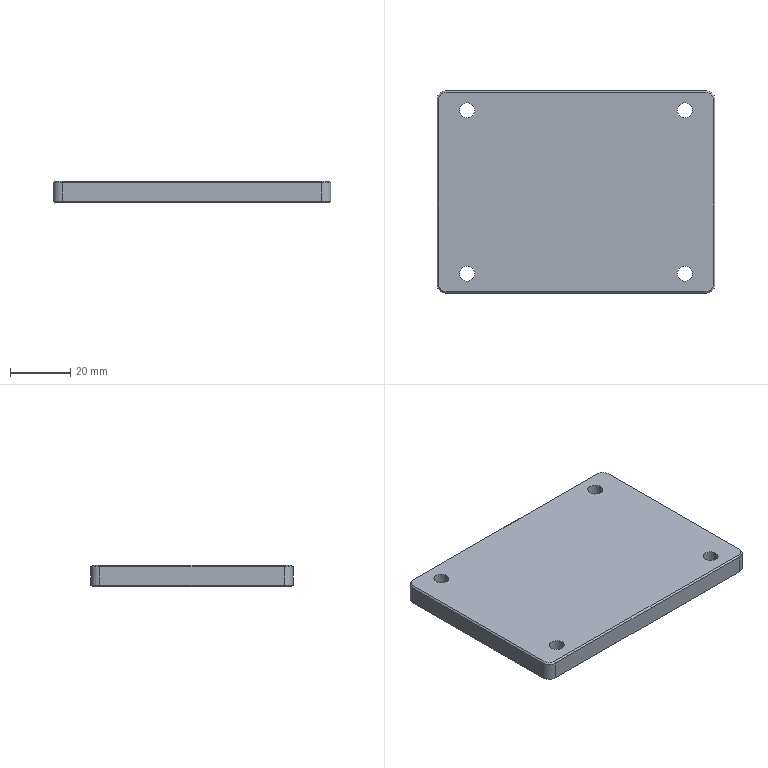Part | SolidWorks | features Chamfer 1, Extrusion 1, Fillet 1, ICE 1, LPattern 1 | 1 solid | 34 faces | box 92 x 67 x 7 mm | volume 42466 mm3 | plane 14 | cylinder 12 | cone 8 | commonest cylinder face diameters 5 x8 6 x4
STEP:
#1=CARTESIAN_POINT('',(38.5,27.,0.));
#2=VERTEX_POINT('',#1);
#3=CARTESIAN_POINT('',(33.5,27.,0.));
#4=VERTEX_POINT('',#3);
#5=CARTESIAN_POINT('',(36.,27.,0.));
#6=DIRECTION('',(0.,0.,-1.));
#7=DIRECTION('',(-1.,0.,0.));
#8=AXIS2_PLACEMENT_3D('',#5,#6,#7);
#9=CIRCLE('',#8,2.5);
#10=EDGE_CURVE('',#2,#4,#9,.T.);
#11=ORIENTED_EDGE('',*,*,#10,.T.);
#12=CARTESIAN_POINT('',(33.5,27.,7.));
#13=VERTEX_POINT('',#12);
#14=CARTESIAN_POINT('',(33.5,27.,-3.));
#15=DIRECTION('',(0.,0.,1.));
#16=VECTOR('',#15,1000.);
#17=LINE('',#14,#16);
#18=EDGE_CURVE('',#4,#13,#17,.T.);
#19=ORIENTED_EDGE('',*,*,#18,.T.);
#20=CARTESIAN_POINT('',(38.5,27.,7.));
#21=VERTEX_POINT('',#20);
#22=CARTESIAN_POINT('',(36.,27.,7.));
#23=DIRECTION('',(0.,0.,1.));
#24=DIRECTION('',(1.,0.,0.));
#25=AXIS2_PLACEMENT_3D('',#22,#23,#24);
#26=CIRCLE('',#25,2.5);
#27=EDGE_CURVE('',#13,#21,#26,.T.);
#28=ORIENTED_EDGE('',*,*,#27,.T.);
#29=CARTESIAN_POINT('',(38.5,27.,-3.));
#30=DIRECTION('',(0.,0.,1.));
#31=VECTOR('',#30,1000.);
#32=LINE('',#29,#31);
#33=EDGE_CURVE('',#2,#21,#32,.T.);
#34=ORIENTED_EDGE('',*,*,#33,.F.);
#35=EDGE_LOOP('',(#11,#19,#28,#34));
#36=FACE_OUTER_BOUND('',#35,.T.);
#37=CARTESIAN_POINT('',(36.,27.,-3.));
#38=DIRECTION('',(0.,0.,1.));
#39=DIRECTION('',(1.,0.,0.));
#40=AXIS2_PLACEMENT_3D('',#37,#38,#39);
#41=CYLINDRICAL_SURFACE('',#40,2.5);
#42=ADVANCED_FACE('',(#36),#41,.F.);
#43=CARTESIAN_POINT('',(-33.5,27.,0.));
#44=VERTEX_POINT('',#43);
#45=CARTESIAN_POINT('',(-38.5,27.,0.));
#46=VERTEX_POINT('',#45);
#47=CARTESIAN_POINT('',(-36.,27.,0.));
#48=DIRECTION('',(0.,0.,-1.));
#49=DIRECTION('',(-1.,0.,0.));
#50=AXIS2_PLACEMENT_3D('',#47,#48,#49);
#51=CIRCLE('',#50,2.5);
#52=EDGE_CURVE('',#44,#46,#51,.T.);
#53=ORIENTED_EDGE('',*,*,#52,.T.);
#54=CARTESIAN_POINT('',(-38.5,27.,7.));
#55=VERTEX_POINT('',#54);
#56=CARTESIAN_POINT('',(-38.5,27.,-3.));
#57=DIRECTION('',(0.,0.,1.));
#58=VECTOR('',#57,1000.);
#59=LINE('',#56,#58);
#60=EDGE_CURVE('',#46,#55,#59,.T.);
#61=ORIENTED_EDGE('',*,*,#60,.T.);
#62=CARTESIAN_POINT('',(-33.5,27.,7.));
#63=VERTEX_POINT('',#62);
#64=CARTESIAN_POINT('',(-36.,27.,7.));
#65=DIRECTION('',(0.,0.,1.));
#66=DIRECTION('',(1.,0.,0.));
#67=AXIS2_PLACEMENT_3D('',#64,#65,#66);
#68=CIRCLE('',#67,2.5);
#69=EDGE_CURVE('',#55,#63,#68,.T.);
#70=ORIENTED_EDGE('',*,*,#69,.T.);
#71=CARTESIAN_POINT('',(-33.5,27.,-3.));
#72=DIRECTION('',(0.,0.,1.));
#73=VECTOR('',#72,1000.);
#74=LINE('',#71,#73);
#75=EDGE_CURVE('',#44,#63,#74,.T.);
#76=ORIENTED_EDGE('',*,*,#75,.F.);
#77=EDGE_LOOP('',(#53,#61,#70,#76));
#78=FACE_OUTER_BOUND('',#77,.T.);
#79=CARTESIAN_POINT('',(-36.,27.,-3.));
#80=DIRECTION('',(0.,0.,1.));
#81=DIRECTION('',(1.,0.,0.));
#82=AXIS2_PLACEMENT_3D('',#79,#80,#81);
#83=CYLINDRICAL_SURFACE('',#82,2.5);
#84=ADVANCED_FACE('',(#78),#83,.F.);
#85=CARTESIAN_POINT('',(-33.5,-27.,0.));
#86=VERTEX_POINT('',#85);
#87=CARTESIAN_POINT('',(-38.5,-27.,0.));
#88=VERTEX_POINT('',#87);
#89=CARTESIAN_POINT('',(-36.,-27.,0.));
#90=DIRECTION('',(0.,0.,-1.));
#91=DIRECTION('',(-1.,0.,0.));
#92=AXIS2_PLACEMENT_3D('',#89,#90,#91);
#93=CIRCLE('',#92,2.5);
#94=EDGE_CURVE('',#86,#88,#93,.T.);
#95=ORIENTED_EDGE('',*,*,#94,.T.);
#96=CARTESIAN_POINT('',(-38.5,-27.,7.));
#97=VERTEX_POINT('',#96);
#98=CARTESIAN_POINT('',(-38.5,-27.,-3.));
#99=DIRECTION('',(0.,0.,1.));
#100=VECTOR('',#99,1000.);
#101=LINE('',#98,#100);
#102=EDGE_CURVE('',#88,#97,#101,.T.);
#103=ORIENTED_EDGE('',*,*,#102,.T.);
#104=CARTESIAN_POINT('',(-33.5,-27.,7.));
#105=VERTEX_POINT('',#104);
#106=CARTESIAN_POINT('',(-36.,-27.,7.));
#107=DIRECTION('',(0.,0.,1.));
#108=DIRECTION('',(1.,0.,0.));
#109=AXIS2_PLACEMENT_3D('',#106,#107,#108);
#110=CIRCLE('',#109,2.5);
#111=EDGE_CURVE('',#97,#105,#110,.T.);
#112=ORIENTED_EDGE('',*,*,#111,.T.);
#113=CARTESIAN_POINT('',(-33.5,-27.,-3.));
#114=DIRECTION('',(0.,0.,1.));
#115=VECTOR('',#114,1000.);
#116=LINE('',#113,#115);
#117=EDGE_CURVE('',#86,#105,#116,.T.);
#118=ORIENTED_EDGE('',*,*,#117,.F.);
#119=EDGE_LOOP('',(#95,#103,#112,#118));
#120=FACE_OUTER_BOUND('',#119,.T.);
#121=CARTESIAN_POINT('',(-36.,-27.,-3.));
#122=DIRECTION('',(0.,0.,1.));
#123=DIRECTION('',(1.,0.,0.));
#124=AXIS2_PLACEMENT_3D('',#121,#122,#123);
#125=CYLINDRICAL_SURFACE('',#124,2.5);
#126=ADVANCED_FACE('',(#120),#125,.F.);
#127=CARTESIAN_POINT('',(38.5,-27.,0.));
#128=VERTEX_POINT('',#127);
#129=CARTESIAN_POINT('',(33.5,-27.,0.));
#130=VERTEX_POINT('',#129);
#131=CARTESIAN_POINT('',(36.,-27.,0.));
#132=DIRECTION('',(0.,0.,-1.));
#133=DIRECTION('',(-1.,0.,0.));
#134=AXIS2_PLACEMENT_3D('',#131,#132,#133);
#135=CIRCLE('',#134,2.5);
#136=EDGE_CURVE('',#128,#130,#135,.T.);
#137=ORIENTED_EDGE('',*,*,#136,.T.);
#138=CARTESIAN_POINT('',(33.5,-27.,7.));
#139=VERTEX_POINT('',#138);
#140=CARTESIAN_POINT('',(33.5,-27.,-3.));
#141=DIRECTION('',(0.,0.,1.));
#142=VECTOR('',#141,1000.);
#143=LINE('',#140,#142);
#144=EDGE_CURVE('',#130,#139,#143,.T.);
#145=ORIENTED_EDGE('',*,*,#144,.T.);
#146=CARTESIAN_POINT('',(38.5,-27.,7.));
#147=VERTEX_POINT('',#146);
#148=CARTESIAN_POINT('',(36.,-27.,7.));
#149=DIRECTION('',(0.,0.,1.));
#150=DIRECTION('',(1.,0.,0.));
#151=AXIS2_PLACEMENT_3D('',#148,#149,#150);
#152=CIRCLE('',#151,2.5);
#153=EDGE_CURVE('',#139,#147,#152,.T.);
#154=ORIENTED_EDGE('',*,*,#153,.T.);
#155=CARTESIAN_POINT('',(38.5,-27.,-3.));
#156=DIRECTION('',(0.,0.,1.));
#157=VECTOR('',#156,1000.);
#158=LINE('',#155,#157);
#159=EDGE_CURVE('',#128,#147,#158,.T.);
#160=ORIENTED_EDGE('',*,*,#159,.F.);
#161=EDGE_LOOP('',(#137,#145,#154,#160));
#162=FACE_OUTER_BOUND('',#161,.T.);
#163=CARTESIAN_POINT('',(36.,-27.,-3.));
#164=DIRECTION('',(0.,0.,1.));
#165=DIRECTION('',(1.,0.,0.));
#166=AXIS2_PLACEMENT_3D('',#163,#164,#165);
#167=CYLINDRICAL_SURFACE('',#166,2.5);
#168=ADVANCED_FACE('',(#162),#167,.F.);
#169=ORIENTED_EDGE('',*,*,#144,.F.);
#170=CARTESIAN_POINT('',(36.,-27.,0.));
#171=DIRECTION('',(0.,0.,-1.));
#172=DIRECTION('',(-1.,0.,0.));
#173=AXIS2_PLACEMENT_3D('',#170,#171,#172);
#174=CIRCLE('',#173,2.5);
#175=EDGE_CURVE('',#130,#128,#174,.T.);
#176=ORIENTED_EDGE('',*,*,#175,.T.);
#177=ORIENTED_EDGE('',*,*,#159,.T.);
#178=CARTESIAN_POINT('',(36.,-27.,7.));
#179=DIRECTION('',(0.,0.,1.));
#180=DIRECTION('',(1.,0.,0.));
#181=AXIS2_PLACEMENT_3D('',#178,#179,#180);
#182=CIRCLE('',#181,2.5);
#183=EDGE_CURVE('',#147,#139,#182,.T.);
#184=ORIENTED_EDGE('',*,*,#183,.T.);
#185=EDGE_LOOP('',(#169,#176,#177,#184));
#186=FACE_OUTER_BOUND('',#185,.T.);
#187=CARTESIAN_POINT('',(36.,-27.,-3.));
#188=DIRECTION('',(0.,0.,1.));
#189=DIRECTION('',(1.,0.,0.));
#190=AXIS2_PLACEMENT_3D('',#187,#188,#189);
#191=CYLINDRICAL_SURFACE('',#190,2.5);
#192=ADVANCED_FACE('',(#186),#191,.F.);
#193=ORIENTED_EDGE('',*,*,#102,.F.);
#194=CARTESIAN_POINT('',(-36.,-27.,0.));
#195=DIRECTION('',(0.,0.,-1.));
#196=DIRECTION('',(-1.,0.,0.));
#197=AXIS2_PLACEMENT_3D('',#194,#195,#196);
#198=CIRCLE('',#197,2.5);
#199=EDGE_CURVE('',#88,#86,#198,.T.);
#200=ORIENTED_EDGE('',*,*,#199,.T.);
#201=ORIENTED_EDGE('',*,*,#117,.T.);
#202=CARTESIAN_POINT('',(-36.,-27.,7.));
#203=DIRECTION('',(0.,0.,1.));
#204=DIRECTION('',(1.,0.,0.));
#205=AXIS2_PLACEMENT_3D('',#202,#203,#204);
#206=CIRCLE('',#205,2.5);
#207=EDGE_CURVE('',#105,#97,#206,.T.);
#208=ORIENTED_EDGE('',*,*,#207,.T.);
#209=EDGE_LOOP('',(#193,#200,#201,#208));
#210=FACE_OUTER_BOUND('',#209,.T.);
#211=CARTESIAN_POINT('',(-36.,-27.,-3.));
#212=DIRECTION('',(0.,0.,1.));
#213=DIRECTION('',(1.,0.,0.));
#214=AXIS2_PLACEMENT_3D('',#211,#212,#213);
#215=CYLINDRICAL_SURFACE('',#214,2.5);
#216=ADVANCED_FACE('',(#210),#215,.F.);
#217=CARTESIAN_POINT('',(46.,-30.5,6.5));
#218=VERTEX_POINT('',#217);
#219=CARTESIAN_POINT('',(46.,-30.5,0.5));
#220=VERTEX_POINT('',#219);
#221=CARTESIAN_POINT('',(46.,-30.5,7.));
#222=DIRECTION('',(0.,0.,-1.));
#223=VECTOR('',#222,1000.);
#224=LINE('',#221,#223);
#225=EDGE_CURVE('',#218,#220,#224,.T.);
#226=ORIENTED_EDGE('',*,*,#225,.T.);
#227=CARTESIAN_POINT('',(46.,30.5,0.5));
#228=VERTEX_POINT('',#227);
#229=CARTESIAN_POINT('',(46.,30.5,0.5));
#230=DIRECTION('',(0.,1.,0.));
#231=VECTOR('',#230,1000.);
#232=LINE('',#229,#231);
#233=EDGE_CURVE('',#220,#228,#232,.T.);
#234=ORIENTED_EDGE('',*,*,#233,.T.);
#235=CARTESIAN_POINT('',(46.,30.5,6.5));
#236=VERTEX_POINT('',#235);
#237=CARTESIAN_POINT('',(46.,30.5,7.));
#238=DIRECTION('',(0.,0.,1.));
#239=VECTOR('',#238,1000.);
#240=LINE('',#237,#239);
#241=EDGE_CURVE('',#228,#236,#240,.T.);
#242=ORIENTED_EDGE('',*,*,#241,.T.);
#243=CARTESIAN_POINT('',(46.,-33.5,6.5));
#244=DIRECTION('',(0.,-1.,0.));
#245=VECTOR('',#244,1000.);
#246=LINE('',#243,#245);
#247=EDGE_CURVE('',#236,#218,#246,.T.);
#248=ORIENTED_EDGE('',*,*,#247,.T.);
#249=EDGE_LOOP('',(#226,#234,#242,#248));
#250=FACE_OUTER_BOUND('',#249,.T.);
#251=CARTESIAN_POINT('',(46.,-33.5,7.));
#252=DIRECTION('',(-1.,0.,0.));
#253=DIRECTION('',(0.,0.,1.));
#254=AXIS2_PLACEMENT_3D('',#251,#252,#253);
#255=PLANE('',#254);
#256=ADVANCED_FACE('',(#250),#255,.F.);
#257=CARTESIAN_POINT('',(43.,33.5,6.5));
#258=VERTEX_POINT('',#257);
#259=CARTESIAN_POINT('',(43.,33.5,0.5));
#260=VERTEX_POINT('',#259);
#261=CARTESIAN_POINT('',(43.,33.5,7.));
#262=DIRECTION('',(0.,0.,-1.));
#263=VECTOR('',#262,1000.);
#264=LINE('',#261,#263);
#265=EDGE_CURVE('',#258,#260,#264,.T.);
#266=ORIENTED_EDGE('',*,*,#265,.T.);
#267=CARTESIAN_POINT('',(-43.,33.5,0.5));
#268=VERTEX_POINT('',#267);
#269=CARTESIAN_POINT('',(-43.,33.5,0.5));
#270=DIRECTION('',(-1.,0.,0.));
#271=VECTOR('',#270,1000.);
#272=LINE('',#269,#271);
#273=EDGE_CURVE('',#260,#268,#272,.T.);
#274=ORIENTED_EDGE('',*,*,#273,.T.);
#275=CARTESIAN_POINT('',(-43.,33.5,6.5));
#276=VERTEX_POINT('',#275);
#277=CARTESIAN_POINT('',(-43.,33.5,7.));
#278=DIRECTION('',(0.,0.,1.));
#279=VECTOR('',#278,1000.);
#280=LINE('',#277,#279);
#281=EDGE_CURVE('',#268,#276,#280,.T.);
#282=ORIENTED_EDGE('',*,*,#281,.T.);
#283=CARTESIAN_POINT('',(-46.,33.5,6.5));
#284=DIRECTION('',(1.,0.,0.));
#285=VECTOR('',#284,1000.);
#286=LINE('',#283,#285);
#287=EDGE_CURVE('',#276,#258,#286,.T.);
#288=ORIENTED_EDGE('',*,*,#287,.T.);
#289=EDGE_LOOP('',(#266,#274,#282,#288));
#290=FACE_OUTER_BOUND('',#289,.T.);
#291=CARTESIAN_POINT('',(-46.,33.5,7.));
#292=DIRECTION('',(0.,-1.,0.));
#293=DIRECTION('',(0.,0.,-1.));
#294=AXIS2_PLACEMENT_3D('',#291,#292,#293);
#295=PLANE('',#294);
#296=ADVANCED_FACE('',(#290),#295,.F.);
#297=CARTESIAN_POINT('',(-46.,30.5,6.5));
#298=VERTEX_POINT('',#297);
#299=CARTESIAN_POINT('',(-46.,30.5,0.5));
#300=VERTEX_POINT('',#299);
#301=CARTESIAN_POINT('',(-46.,30.5,7.));
#302=DIRECTION('',(0.,0.,-1.));
#303=VECTOR('',#302,1000.);
#304=LINE('',#301,#303);
#305=EDGE_CURVE('',#298,#300,#304,.T.);
#306=ORIENTED_EDGE('',*,*,#305,.T.);
#307=CARTESIAN_POINT('',(-46.,-30.5,0.5));
#308=VERTEX_POINT('',#307);
#309=CARTESIAN_POINT('',(-46.,-30.5,0.5));
#310=DIRECTION('',(0.,-1.,0.));
#311=VECTOR('',#310,1000.);
#312=LINE('',#309,#311);
#313=EDGE_CURVE('',#300,#308,#312,.T.);
#314=ORIENTED_EDGE('',*,*,#313,.T.);
#315=CARTESIAN_POINT('',(-46.,-30.5,6.5));
#316=VERTEX_POINT('',#315);
#317=CARTESIAN_POINT('',(-46.,-30.5,7.));
#318=DIRECTION('',(0.,0.,1.));
#319=VECTOR('',#318,1000.);
#320=LINE('',#317,#319);
#321=EDGE_CURVE('',#308,#316,#320,.T.);
#322=ORIENTED_EDGE('',*,*,#321,.T.);
#323=CARTESIAN_POINT('',(-46.,-33.5,6.5));
#324=DIRECTION('',(0.,1.,0.));
#325=VECTOR('',#324,1000.);
#326=LINE('',#323,#325);
#327=EDGE_CURVE('',#316,#298,#326,.T.);
#328=ORIENTED_EDGE('',*,*,#327,.T.);
#329=EDGE_LOOP('',(#306,#314,#322,#328));
#330=FACE_OUTER_BOUND('',#329,.T.);
#331=CARTESIAN_POINT('',(-46.,-33.5,7.));
#332=DIRECTION('',(1.,0.,0.));
#333=DIRECTION('',(0.,0.,-1.));
#334=AXIS2_PLACEMENT_3D('',#331,#332,#333);
#335=PLANE('',#334);
#336=ADVANCED_FACE('',(#330),#335,.F.);
#337=CARTESIAN_POINT('',(-43.,-33.5,6.5));
#338=VERTEX_POINT('',#337);
#339=CARTESIAN_POINT('',(-43.,-33.5,0.5));
#340=VERTEX_POINT('',#339);
#341=CARTESIAN_POINT('',(-43.,-33.5,7.));
#342=DIRECTION('',(0.,0.,-1.));
#343=VECTOR('',#342,1000.);
#344=LINE('',#341,#343);
#345=EDGE_CURVE('',#338,#340,#344,.T.);
#346=ORIENTED_EDGE('',*,*,#345,.T.);
#347=CARTESIAN_POINT('',(43.,-33.5,0.5));
#348=VERTEX_POINT('',#347);
#349=CARTESIAN_POINT('',(43.,-33.5,0.5));
#350=DIRECTION('',(1.,0.,0.));
#351=VECTOR('',#350,1000.);
#352=LINE('',#349,#351);
#353=EDGE_CURVE('',#340,#348,#352,.T.);
#354=ORIENTED_EDGE('',*,*,#353,.T.);
#355=CARTESIAN_POINT('',(43.,-33.5,6.5));
#356=VERTEX_POINT('',#355);
#357=CARTESIAN_POINT('',(43.,-33.5,7.));
#358=DIRECTION('',(0.,0.,1.));
#359=VECTOR('',#358,1000.);
#360=LINE('',#357,#359);
#361=EDGE_CURVE('',#348,#356,#360,.T.);
#362=ORIENTED_EDGE('',*,*,#361,.T.);
#363=CARTESIAN_POINT('',(-46.,-33.5,6.5));
#364=DIRECTION('',(-1.,0.,0.));
#365=VECTOR('',#364,1000.);
#366=LINE('',#363,#365);
#367=EDGE_CURVE('',#356,#338,#366,.T.);
#368=ORIENTED_EDGE('',*,*,#367,.T.);
#369=EDGE_LOOP('',(#346,#354,#362,#368));
#370=FACE_OUTER_BOUND('',#369,.T.);
#371=CARTESIAN_POINT('',(-46.,-33.5,7.));
#372=DIRECTION('',(0.,1.,0.));
#373=DIRECTION('',(0.,0.,1.));
#374=AXIS2_PLACEMENT_3D('',#371,#372,#373);
#375=PLANE('',#374);
#376=ADVANCED_FACE('',(#370),#375,.F.);
#377=CARTESIAN_POINT('',(43.,-33.,7.));
#378=VERTEX_POINT('',#377);
#379=CARTESIAN_POINT('',(45.5,-30.5,7.));
#380=VERTEX_POINT('',#379);
#381=CARTESIAN_POINT('',(43.,-30.5,7.));
#382=DIRECTION('',(0.,0.,1.));
#383=DIRECTION('',(-1.,0.,0.));
#384=AXIS2_PLACEMENT_3D('',#381,#382,#383);
#385=CIRCLE('',#384,2.5);
#386=EDGE_CURVE('',#378,#380,#385,.T.);
#387=ORIENTED_EDGE('',*,*,#386,.T.);
#388=CARTESIAN_POINT('',(45.5,30.5,7.));
#389=VERTEX_POINT('',#388);
#390=CARTESIAN_POINT('',(45.5,0.,7.));
#391=DIRECTION('',(0.,1.,0.));
#392=VECTOR('',#391,1000.);
#393=LINE('',#390,#392);
#394=EDGE_CURVE('',#380,#389,#393,.T.);
#395=ORIENTED_EDGE('',*,*,#394,.T.);
#396=CARTESIAN_POINT('',(43.,33.,7.));
#397=VERTEX_POINT('',#396);
#398=CARTESIAN_POINT('',(43.,30.5,7.));
#399=DIRECTION('',(0.,0.,1.));
#400=DIRECTION('',(-1.,0.,0.));
#401=AXIS2_PLACEMENT_3D('',#398,#399,#400);
#402=CIRCLE('',#401,2.5);
#403=EDGE_CURVE('',#389,#397,#402,.T.);
#404=ORIENTED_EDGE('',*,*,#403,.T.);
#405=CARTESIAN_POINT('',(-43.,33.,7.));
#406=VERTEX_POINT('',#405);
#407=CARTESIAN_POINT('',(0.,33.,7.));
#408=DIRECTION('',(-1.,0.,0.));
#409=VECTOR('',#408,1000.);
#410=LINE('',#407,#409);
#411=EDGE_CURVE('',#397,#406,#410,.T.);
#412=ORIENTED_EDGE('',*,*,#411,.T.);
#413=CARTESIAN_POINT('',(-45.5,30.5,7.));
#414=VERTEX_POINT('',#413);
#415=CARTESIAN_POINT('',(-43.,30.5,7.));
#416=DIRECTION('',(0.,0.,1.));
#417=DIRECTION('',(-1.,0.,0.));
#418=AXIS2_PLACEMENT_3D('',#415,#416,#417);
#419=CIRCLE('',#418,2.5);
#420=EDGE_CURVE('',#406,#414,#419,.T.);
#421=ORIENTED_EDGE('',*,*,#420,.T.);
#422=CARTESIAN_POINT('',(-45.5,-30.5,7.));
#423=VERTEX_POINT('',#422);
#424=CARTESIAN_POINT('',(-45.5,0.,7.));
#425=DIRECTION('',(0.,-1.,0.));
#426=VECTOR('',#425,1000.);
#427=LINE('',#424,#426);
#428=EDGE_CURVE('',#414,#423,#427,.T.);
#429=ORIENTED_EDGE('',*,*,#428,.T.);
#430=CARTESIAN_POINT('',(-43.,-33.,7.));
#431=VERTEX_POINT('',#430);
#432=CARTESIAN_POINT('',(-43.,-30.5,7.));
#433=DIRECTION('',(0.,0.,1.));
#434=DIRECTION('',(-1.,0.,0.));
#435=AXIS2_PLACEMENT_3D('',#432,#433,#434);
#436=CIRCLE('',#435,2.5);
#437=EDGE_CURVE('',#423,#431,#436,.T.);
#438=ORIENTED_EDGE('',*,*,#437,.T.);
#439=CARTESIAN_POINT('',(0.,-33.,7.));
#440=DIRECTION('',(1.,0.,0.));
#441=VECTOR('',#440,1000.);
#442=LINE('',#439,#441);
#443=EDGE_CURVE('',#431,#378,#442,.T.);
#444=ORIENTED_EDGE('',*,*,#443,.T.);
#445=EDGE_LOOP('',(#387,#395,#404,#412,#421,#429,#438,#444));
#446=FACE_OUTER_BOUND('',#445,.T.);
#447=CARTESIAN_POINT('',(36.,27.,7.));
#448=DIRECTION('',(0.,0.,1.));
#449=DIRECTION('',(1.,0.,0.));
#450=AXIS2_PLACEMENT_3D('',#447,#448,#449);
#451=CIRCLE('',#450,2.5);
#452=EDGE_CURVE('',#21,#13,#451,.T.);
#453=ORIENTED_EDGE('',*,*,#452,.F.);
#454=ORIENTED_EDGE('',*,*,#27,.F.);
#455=EDGE_LOOP('',(#453,#454));
#456=FACE_BOUND('',#455,.T.);
#457=CARTESIAN_POINT('',(-36.,27.,7.));
#458=DIRECTION('',(0.,0.,1.));
#459=DIRECTION('',(1.,0.,0.));
#460=AXIS2_PLACEMENT_3D('',#457,#458,#459);
#461=CIRCLE('',#460,2.5);
#462=EDGE_CURVE('',#63,#55,#461,.T.);
#463=ORIENTED_EDGE('',*,*,#462,.F.);
#464=ORIENTED_EDGE('',*,*,#69,.F.);
#465=EDGE_LOOP('',(#463,#464));
#466=FACE_BOUND('',#465,.T.);
#467=ORIENTED_EDGE('',*,*,#207,.F.);
#468=ORIENTED_EDGE('',*,*,#111,.F.);
#469=EDGE_LOOP('',(#467,#468));
#470=FACE_BOUND('',#469,.T.);
#471=ORIENTED_EDGE('',*,*,#183,.F.);
#472=ORIENTED_EDGE('',*,*,#153,.F.);
#473=EDGE_LOOP('',(#471,#472));
#474=FACE_BOUND('',#473,.T.);
#475=CARTESIAN_POINT('',(0.,0.,7.));
#476=DIRECTION('',(0.,0.,-1.));
#477=DIRECTION('',(-1.,0.,0.));
#478=AXIS2_PLACEMENT_3D('',#475,#476,#477);
#479=PLANE('',#478);
#480=ADVANCED_FACE('',(#446,#456,#466,#470,#474),#479,.F.);
#481=CARTESIAN_POINT('',(43.,33.,0.));
#482=VERTEX_POINT('',#481);
#483=CARTESIAN_POINT('',(45.5,30.5,0.));
#484=VERTEX_POINT('',#483);
#485=CARTESIAN_POINT('',(43.,30.5,0.));
#486=DIRECTION('',(0.,0.,-1.));
#487=DIRECTION('',(-1.,0.,0.));
#488=AXIS2_PLACEMENT_3D('',#485,#486,#487);
#489=CIRCLE('',#488,2.5);
#490=EDGE_CURVE('',#482,#484,#489,.T.);
#491=ORIENTED_EDGE('',*,*,#490,.T.);
#492=CARTESIAN_POINT('',(45.5,-30.5,0.));
#493=VERTEX_POINT('',#492);
#494=CARTESIAN_POINT('',(45.5,-30.5,0.));
#495=DIRECTION('',(0.,-1.,0.));
#496=VECTOR('',#495,1000.);
#497=LINE('',#494,#496);
#498=EDGE_CURVE('',#484,#493,#497,.T.);
#499=ORIENTED_EDGE('',*,*,#498,.T.);
#500=CARTESIAN_POINT('',(43.,-33.,0.));
#501=VERTEX_POINT('',#500);
#502=CARTESIAN_POINT('',(43.,-30.5,0.));
#503=DIRECTION('',(0.,0.,-1.));
#504=DIRECTION('',(-1.,0.,0.));
#505=AXIS2_PLACEMENT_3D('',#502,#503,#504);
#506=CIRCLE('',#505,2.5);
#507=EDGE_CURVE('',#493,#501,#506,.T.);
#508=ORIENTED_EDGE('',*,*,#507,.T.);
#509=CARTESIAN_POINT('',(-43.,-33.,0.));
#510=VERTEX_POINT('',#509);
#511=CARTESIAN_POINT('',(-43.,-33.,0.));
#512=DIRECTION('',(-1.,0.,0.));
#513=VECTOR('',#512,1000.);
#514=LINE('',#511,#513);
#515=EDGE_CURVE('',#501,#510,#514,.T.);
#516=ORIENTED_EDGE('',*,*,#515,.T.);
#517=CARTESIAN_POINT('',(-45.5,-30.5,0.));
#518=VERTEX_POINT('',#517);
#519=CARTESIAN_POINT('',(-43.,-30.5,0.));
#520=DIRECTION('',(0.,0.,-1.));
#521=DIRECTION('',(-1.,0.,0.));
#522=AXIS2_PLACEMENT_3D('',#519,#520,#521);
#523=CIRCLE('',#522,2.5);
#524=EDGE_CURVE('',#510,#518,#523,.T.);
#525=ORIENTED_EDGE('',*,*,#524,.T.);
#526=CARTESIAN_POINT('',(-45.5,30.5,0.));
#527=VERTEX_POINT('',#526);
#528=CARTESIAN_POINT('',(-45.5,30.5,0.));
#529=DIRECTION('',(0.,1.,0.));
#530=VECTOR('',#529,1000.);
#531=LINE('',#528,#530);
#532=EDGE_CURVE('',#518,#527,#531,.T.);
#533=ORIENTED_EDGE('',*,*,#532,.T.);
#534=CARTESIAN_POINT('',(-43.,33.,0.));
#535=VERTEX_POINT('',#534);
#536=CARTESIAN_POINT('',(-43.,30.5,0.));
#537=DIRECTION('',(0.,0.,-1.));
#538=DIRECTION('',(-1.,0.,0.));
#539=AXIS2_PLACEMENT_3D('',#536,#537,#538);
#540=CIRCLE('',#539,2.5);
#541=EDGE_CURVE('',#527,#535,#540,.T.);
#542=ORIENTED_EDGE('',*,*,#541,.T.);
#543=CARTESIAN_POINT('',(43.,33.,0.));
#544=DIRECTION('',(1.,0.,0.));
#545=VECTOR('',#544,1000.);
#546=LINE('',#543,#545);
#547=EDGE_CURVE('',#535,#482,#546,.T.);
#548=ORIENTED_EDGE('',*,*,#547,.T.);
#549=EDGE_LOOP('',(#491,#499,#508,#516,#525,#533,#542,#548));
#550=FACE_OUTER_BOUND('',#549,.T.);
#551=ORIENTED_EDGE('',*,*,#10,.F.);
#552=CARTESIAN_POINT('',(36.,27.,0.));
#553=DIRECTION('',(0.,0.,-1.));
#554=DIRECTION('',(-1.,0.,0.));
#555=AXIS2_PLACEMENT_3D('',#552,#553,#554);
#556=CIRCLE('',#555,2.5);
#557=EDGE_CURVE('',#4,#2,#556,.T.);
#558=ORIENTED_EDGE('',*,*,#557,.F.);
#559=EDGE_LOOP('',(#551,#558));
#560=FACE_BOUND('',#559,.T.);
#561=ORIENTED_EDGE('',*,*,#52,.F.);
#562=CARTESIAN_POINT('',(-36.,27.,0.));
#563=DIRECTION('',(0.,0.,-1.));
#564=DIRECTION('',(-1.,0.,0.));
#565=AXIS2_PLACEMENT_3D('',#562,#563,#564);
#566=CIRCLE('',#565,2.5);
#567=EDGE_CURVE('',#46,#44,#566,.T.);
#568=ORIENTED_EDGE('',*,*,#567,.F.);
#569=EDGE_LOOP('',(#561,#568));
#570=FACE_BOUND('',#569,.T.);
#571=ORIENTED_EDGE('',*,*,#94,.F.);
#572=ORIENTED_EDGE('',*,*,#199,.F.);
#573=EDGE_LOOP('',(#571,#572));
#574=FACE_BOUND('',#573,.T.);
#575=ORIENTED_EDGE('',*,*,#136,.F.);
#576=ORIENTED_EDGE('',*,*,#175,.F.);
#577=EDGE_LOOP('',(#575,#576));
#578=FACE_BOUND('',#577,.T.);
#579=CARTESIAN_POINT('',(0.,0.,0.));
#580=DIRECTION('',(0.,0.,-1.));
#581=DIRECTION('',(-1.,0.,0.));
#582=AXIS2_PLACEMENT_3D('',#579,#580,#581);
#583=PLANE('',#582);
#584=ADVANCED_FACE('',(#550,#560,#570,#574,#578),#583,.T.);
#585=ORIENTED_EDGE('',*,*,#361,.F.);
#586=CARTESIAN_POINT('',(43.,-30.5,0.5));
#587=DIRECTION('',(0.,0.,1.));
#588=DIRECTION('',(-1.,0.,0.));
#589=AXIS2_PLACEMENT_3D('',#586,#587,#588);
#590=CIRCLE('',#589,3.);
#591=EDGE_CURVE('',#348,#220,#590,.T.);
#592=ORIENTED_EDGE('',*,*,#591,.T.);
#593=ORIENTED_EDGE('',*,*,#225,.F.);
#594=CARTESIAN_POINT('',(43.,-30.5,6.5));
#595=DIRECTION('',(0.,0.,-1.));
#596=DIRECTION('',(-1.,0.,0.));
#597=AXIS2_PLACEMENT_3D('',#594,#595,#596);
#598=CIRCLE('',#597,3.);
#599=EDGE_CURVE('',#218,#356,#598,.T.);
#600=ORIENTED_EDGE('',*,*,#599,.T.);
#601=EDGE_LOOP('',(#585,#592,#593,#600));
#602=FACE_OUTER_BOUND('',#601,.T.);
#603=CARTESIAN_POINT('',(43.,-30.5,7.));
#604=DIRECTION('',(0.,0.,-1.));
#605=DIRECTION('',(-1.,0.,0.));
#606=AXIS2_PLACEMENT_3D('',#603,#604,#605);
#607=CYLINDRICAL_SURFACE('',#606,3.);
#608=ADVANCED_FACE('',(#602),#607,.T.);
#609=ORIENTED_EDGE('',*,*,#321,.F.);
#610=CARTESIAN_POINT('',(-43.,-30.5,0.5));
#611=DIRECTION('',(0.,0.,1.));
#612=DIRECTION('',(-1.,0.,0.));
#613=AXIS2_PLACEMENT_3D('',#610,#611,#612);
#614=CIRCLE('',#613,3.);
#615=EDGE_CURVE('',#308,#340,#614,.T.);
#616=ORIENTED_EDGE('',*,*,#615,.T.);
#617=ORIENTED_EDGE('',*,*,#345,.F.);
#618=CARTESIAN_POINT('',(-43.,-30.5,6.5));
#619=DIRECTION('',(0.,0.,-1.));
#620=DIRECTION('',(-1.,0.,0.));
#621=AXIS2_PLACEMENT_3D('',#618,#619,#620);
#622=CIRCLE('',#621,3.);
#623=EDGE_CURVE('',#338,#316,#622,.T.);
#624=ORIENTED_EDGE('',*,*,#623,.T.);
#625=EDGE_LOOP('',(#609,#616,#617,#624));
#626=FACE_OUTER_BOUND('',#625,.T.);
#627=CARTESIAN_POINT('',(-43.,-30.5,7.));
#628=DIRECTION('',(0.,0.,-1.));
#629=DIRECTION('',(-1.,0.,0.));
#630=AXIS2_PLACEMENT_3D('',#627,#628,#629);
#631=CYLINDRICAL_SURFACE('',#630,3.);
#632=ADVANCED_FACE('',(#626),#631,.T.);
#633=ORIENTED_EDGE('',*,*,#241,.F.);
#634=CARTESIAN_POINT('',(43.,30.5,0.5));
#635=DIRECTION('',(0.,0.,1.));
#636=DIRECTION('',(-1.,0.,0.));
#637=AXIS2_PLACEMENT_3D('',#634,#635,#636);
#638=CIRCLE('',#637,3.);
#639=EDGE_CURVE('',#228,#260,#638,.T.);
#640=ORIENTED_EDGE('',*,*,#639,.T.);
#641=ORIENTED_EDGE('',*,*,#265,.F.);
#642=CARTESIAN_POINT('',(43.,30.5,6.5));
#643=DIRECTION('',(0.,0.,-1.));
#644=DIRECTION('',(-1.,0.,0.));
#645=AXIS2_PLACEMENT_3D('',#642,#643,#644);
#646=CIRCLE('',#645,3.);
#647=EDGE_CURVE('',#258,#236,#646,.T.);
#648=ORIENTED_EDGE('',*,*,#647,.T.);
#649=EDGE_LOOP('',(#633,#640,#641,#648));
#650=FACE_OUTER_BOUND('',#649,.T.);
#651=CARTESIAN_POINT('',(43.,30.5,7.));
#652=DIRECTION('',(0.,0.,-1.));
#653=DIRECTION('',(-1.,0.,0.));
#654=AXIS2_PLACEMENT_3D('',#651,#652,#653);
#655=CYLINDRICAL_SURFACE('',#654,3.);
#656=ADVANCED_FACE('',(#650),#655,.T.);
#657=ORIENTED_EDGE('',*,*,#281,.F.);
#658=CARTESIAN_POINT('',(-43.,30.5,0.5));
#659=DIRECTION('',(0.,0.,1.));
#660=DIRECTION('',(-1.,0.,0.));
#661=AXIS2_PLACEMENT_3D('',#658,#659,#660);
#662=CIRCLE('',#661,3.);
#663=EDGE_CURVE('',#268,#300,#662,.T.);
#664=ORIENTED_EDGE('',*,*,#663,.T.);
#665=ORIENTED_EDGE('',*,*,#305,.F.);
#666=CARTESIAN_POINT('',(-43.,30.5,6.5));
#667=DIRECTION('',(0.,0.,-1.));
#668=DIRECTION('',(-1.,0.,0.));
#669=AXIS2_PLACEMENT_3D('',#666,#667,#668);
#670=CIRCLE('',#669,3.);
#671=EDGE_CURVE('',#298,#276,#670,.T.);
#672=ORIENTED_EDGE('',*,*,#671,.T.);
#673=EDGE_LOOP('',(#657,#664,#665,#672));
#674=FACE_OUTER_BOUND('',#673,.T.);
#675=CARTESIAN_POINT('',(-43.,30.5,7.));
#676=DIRECTION('',(0.,0.,-1.));
#677=DIRECTION('',(-1.,0.,0.));
#678=AXIS2_PLACEMENT_3D('',#675,#676,#677);
#679=CYLINDRICAL_SURFACE('',#678,3.);
#680=ADVANCED_FACE('',(#674),#679,.T.);
#681=ORIENTED_EDGE('',*,*,#60,.F.);
#682=ORIENTED_EDGE('',*,*,#567,.T.);
#683=ORIENTED_EDGE('',*,*,#75,.T.);
#684=ORIENTED_EDGE('',*,*,#462,.T.);
#685=EDGE_LOOP('',(#681,#682,#683,#684));
#686=FACE_OUTER_BOUND('',#685,.T.);
#687=CARTESIAN_POINT('',(-36.,27.,-3.));
#688=DIRECTION('',(0.,0.,1.));
#689=DIRECTION('',(1.,0.,0.));
#690=AXIS2_PLACEMENT_3D('',#687,#688,#689);
#691=CYLINDRICAL_SURFACE('',#690,2.5);
#692=ADVANCED_FACE('',(#686),#691,.F.);
#693=ORIENTED_EDGE('',*,*,#18,.F.);
#694=ORIENTED_EDGE('',*,*,#557,.T.);
#695=ORIENTED_EDGE('',*,*,#33,.T.);
#696=ORIENTED_EDGE('',*,*,#452,.T.);
#697=EDGE_LOOP('',(#693,#694,#695,#696));
#698=FACE_OUTER_BOUND('',#697,.T.);
#699=CARTESIAN_POINT('',(36.,27.,-3.));
#700=DIRECTION('',(0.,0.,1.));
#701=DIRECTION('',(1.,0.,0.));
#702=AXIS2_PLACEMENT_3D('',#699,#700,#701);
#703=CYLINDRICAL_SURFACE('',#702,2.5);
#704=ADVANCED_FACE('',(#698),#703,.F.);
#705=CARTESIAN_POINT('',(-45.5,30.5,0.));
#706=DIRECTION('',(-0.7071,0.,0.7071));
#707=VECTOR('',#706,1000.);
#708=LINE('',#705,#707);
#709=EDGE_CURVE('',#527,#300,#708,.T.);
#710=ORIENTED_EDGE('',*,*,#709,.F.);
#711=ORIENTED_EDGE('',*,*,#532,.F.);
#712=CARTESIAN_POINT('',(-46.,-30.5,0.5));
#713=DIRECTION('',(0.7071,0.,-0.7071));
#714=VECTOR('',#713,1000.);
#715=LINE('',#712,#714);
#716=EDGE_CURVE('',#308,#518,#715,.T.);
#717=ORIENTED_EDGE('',*,*,#716,.F.);
#718=ORIENTED_EDGE('',*,*,#313,.F.);
#719=EDGE_LOOP('',(#710,#711,#717,#718));
#720=FACE_OUTER_BOUND('',#719,.T.);
#721=CARTESIAN_POINT('',(-46.,-33.5,0.5));
#722=DIRECTION('',(-0.7071,0.,-0.7071));
#723=DIRECTION('',(0.,1.,0.));
#724=AXIS2_PLACEMENT_3D('',#721,#722,#723);
#725=PLANE('',#724);
#726=ADVANCED_FACE('',(#720),#725,.T.);
#727=ORIENTED_EDGE('',*,*,#716,.T.);
#728=ORIENTED_EDGE('',*,*,#524,.F.);
#729=CARTESIAN_POINT('',(-43.,-33.5,0.5));
#730=DIRECTION('',(0.,0.7071,-0.7071));
#731=VECTOR('',#730,1000.);
#732=LINE('',#729,#731);
#733=EDGE_CURVE('',#340,#510,#732,.T.);
#734=ORIENTED_EDGE('',*,*,#733,.F.);
#735=ORIENTED_EDGE('',*,*,#615,.F.);
#736=EDGE_LOOP('',(#727,#728,#734,#735));
#737=FACE_OUTER_BOUND('',#736,.T.);
#738=CARTESIAN_POINT('',(-43.,-30.5,0.));
#739=DIRECTION('',(0.,0.,1.));
#740=DIRECTION('',(1.,0.,0.));
#741=AXIS2_PLACEMENT_3D('',#738,#739,#740);
#742=CONICAL_SURFACE('',#741,2.5,0.7854);
#743=ADVANCED_FACE('',(#737),#742,.T.);
#744=ORIENTED_EDGE('',*,*,#709,.T.);
#745=ORIENTED_EDGE('',*,*,#663,.F.);
#746=CARTESIAN_POINT('',(-43.,33.,0.));
#747=DIRECTION('',(0.,0.7071,0.7071));
#748=VECTOR('',#747,1000.);
#749=LINE('',#746,#748);
#750=EDGE_CURVE('',#535,#268,#749,.T.);
#751=ORIENTED_EDGE('',*,*,#750,.F.);
#752=ORIENTED_EDGE('',*,*,#541,.F.);
#753=EDGE_LOOP('',(#744,#745,#751,#752));
#754=FACE_OUTER_BOUND('',#753,.T.);
#755=CARTESIAN_POINT('',(-43.,30.5,0.));
#756=DIRECTION('',(0.,0.,1.));
#757=DIRECTION('',(1.,0.,0.));
#758=AXIS2_PLACEMENT_3D('',#755,#756,#757);
#759=CONICAL_SURFACE('',#758,2.5,0.7854);
#760=ADVANCED_FACE('',(#754),#759,.T.);
#761=ORIENTED_EDGE('',*,*,#733,.T.);
#762=ORIENTED_EDGE('',*,*,#515,.F.);
#763=CARTESIAN_POINT('',(43.,-33.5,0.5));
#764=DIRECTION('',(0.,0.7071,-0.7071));
#765=VECTOR('',#764,1000.);
#766=LINE('',#763,#765);
#767=EDGE_CURVE('',#348,#501,#766,.T.);
#768=ORIENTED_EDGE('',*,*,#767,.F.);
#769=ORIENTED_EDGE('',*,*,#353,.F.);
#770=EDGE_LOOP('',(#761,#762,#768,#769));
#771=FACE_OUTER_BOUND('',#770,.T.);
#772=CARTESIAN_POINT('',(-46.,-33.5,0.5));
#773=DIRECTION('',(0.,-0.7071,-0.7071));
#774=DIRECTION('',(-1.,0.,0.));
#775=AXIS2_PLACEMENT_3D('',#772,#773,#774);
#776=PLANE('',#775);
#777=ADVANCED_FACE('',(#771),#776,.T.);
#778=ORIENTED_EDGE('',*,*,#750,.T.);
#779=ORIENTED_EDGE('',*,*,#273,.F.);
#780=CARTESIAN_POINT('',(43.,33.,0.));
#781=DIRECTION('',(0.,0.7071,0.7071));
#782=VECTOR('',#781,1000.);
#783=LINE('',#780,#782);
#784=EDGE_CURVE('',#482,#260,#783,.T.);
#785=ORIENTED_EDGE('',*,*,#784,.F.);
#786=ORIENTED_EDGE('',*,*,#547,.F.);
#787=EDGE_LOOP('',(#778,#779,#785,#786));
#788=FACE_OUTER_BOUND('',#787,.T.);
#789=CARTESIAN_POINT('',(-46.,33.5,0.5));
#790=DIRECTION('',(0.,0.7071,-0.7071));
#791=DIRECTION('',(1.,0.,0.));
#792=AXIS2_PLACEMENT_3D('',#789,#790,#791);
#793=PLANE('',#792);
#794=ADVANCED_FACE('',(#788),#793,.T.);
#795=ORIENTED_EDGE('',*,*,#767,.T.);
#796=ORIENTED_EDGE('',*,*,#507,.F.);
#797=CARTESIAN_POINT('',(46.,-30.5,0.5));
#798=DIRECTION('',(-0.7071,0.,-0.7071));
#799=VECTOR('',#798,1000.);
#800=LINE('',#797,#799);
#801=EDGE_CURVE('',#220,#493,#800,.T.);
#802=ORIENTED_EDGE('',*,*,#801,.F.);
#803=ORIENTED_EDGE('',*,*,#591,.F.);
#804=EDGE_LOOP('',(#795,#796,#802,#803));
#805=FACE_OUTER_BOUND('',#804,.T.);
#806=CARTESIAN_POINT('',(43.,-30.5,0.));
#807=DIRECTION('',(0.,0.,1.));
#808=DIRECTION('',(1.,0.,0.));
#809=AXIS2_PLACEMENT_3D('',#806,#807,#808);
#810=CONICAL_SURFACE('',#809,2.5,0.7854);
#811=ADVANCED_FACE('',(#805),#810,.T.);
#812=ORIENTED_EDGE('',*,*,#784,.T.);
#813=ORIENTED_EDGE('',*,*,#639,.F.);
#814=CARTESIAN_POINT('',(45.5,30.5,0.));
#815=DIRECTION('',(0.7071,0.,0.7071));
#816=VECTOR('',#815,1000.);
#817=LINE('',#814,#816);
#818=EDGE_CURVE('',#484,#228,#817,.T.);
#819=ORIENTED_EDGE('',*,*,#818,.F.);
#820=ORIENTED_EDGE('',*,*,#490,.F.);
#821=EDGE_LOOP('',(#812,#813,#819,#820));
#822=FACE_OUTER_BOUND('',#821,.T.);
#823=CARTESIAN_POINT('',(43.,30.5,0.));
#824=DIRECTION('',(0.,0.,1.));
#825=DIRECTION('',(1.,0.,0.));
#826=AXIS2_PLACEMENT_3D('',#823,#824,#825);
#827=CONICAL_SURFACE('',#826,2.5,0.7854);
#828=ADVANCED_FACE('',(#822),#827,.T.);
#829=ORIENTED_EDGE('',*,*,#801,.T.);
#830=ORIENTED_EDGE('',*,*,#498,.F.);
#831=ORIENTED_EDGE('',*,*,#818,.T.);
#832=ORIENTED_EDGE('',*,*,#233,.F.);
#833=EDGE_LOOP('',(#829,#830,#831,#832));
#834=FACE_OUTER_BOUND('',#833,.T.);
#835=CARTESIAN_POINT('',(46.,-33.5,0.5));
#836=DIRECTION('',(0.7071,0.,-0.7071));
#837=DIRECTION('',(0.,-1.,0.));
#838=AXIS2_PLACEMENT_3D('',#835,#836,#837);
#839=PLANE('',#838);
#840=ADVANCED_FACE('',(#834),#839,.T.);
#841=CARTESIAN_POINT('',(-46.,30.5,6.5));
#842=DIRECTION('',(0.7071,0.,0.7071));
#843=VECTOR('',#842,1000.);
#844=LINE('',#841,#843);
#845=EDGE_CURVE('',#298,#414,#844,.T.);
#846=ORIENTED_EDGE('',*,*,#845,.F.);
#847=ORIENTED_EDGE('',*,*,#327,.F.);
#848=CARTESIAN_POINT('',(-45.5,-30.5,7.));
#849=DIRECTION('',(-0.7071,0.,-0.7071));
#850=VECTOR('',#849,1000.);
#851=LINE('',#848,#850);
#852=EDGE_CURVE('',#423,#316,#851,.T.);
#853=ORIENTED_EDGE('',*,*,#852,.F.);
#854=ORIENTED_EDGE('',*,*,#428,.F.);
#855=EDGE_LOOP('',(#846,#847,#853,#854));
#856=FACE_OUTER_BOUND('',#855,.T.);
#857=CARTESIAN_POINT('',(-45.5,0.,7.));
#858=DIRECTION('',(0.7071,0.,-0.7071));
#859=DIRECTION('',(0.,-1.,0.));
#860=AXIS2_PLACEMENT_3D('',#857,#858,#859);
#861=PLANE('',#860);
#862=ADVANCED_FACE('',(#856),#861,.F.);
#863=ORIENTED_EDGE('',*,*,#852,.T.);
#864=ORIENTED_EDGE('',*,*,#623,.F.);
#865=CARTESIAN_POINT('',(-43.,-33.,7.));
#866=DIRECTION('',(0.,-0.7071,-0.7071));
#867=VECTOR('',#866,1000.);
#868=LINE('',#865,#867);
#869=EDGE_CURVE('',#431,#338,#868,.T.);
#870=ORIENTED_EDGE('',*,*,#869,.F.);
#871=ORIENTED_EDGE('',*,*,#437,.F.);
#872=EDGE_LOOP('',(#863,#864,#870,#871));
#873=FACE_OUTER_BOUND('',#872,.T.);
#874=CARTESIAN_POINT('',(-43.,-30.5,7.));
#875=DIRECTION('',(0.,0.,-1.));
#876=DIRECTION('',(-1.,0.,0.));
#877=AXIS2_PLACEMENT_3D('',#874,#875,#876);
#878=CONICAL_SURFACE('',#877,2.5,0.7854);
#879=ADVANCED_FACE('',(#873),#878,.T.);
#880=ORIENTED_EDGE('',*,*,#845,.T.);
#881=ORIENTED_EDGE('',*,*,#420,.F.);
#882=CARTESIAN_POINT('',(-43.,33.5,6.5));
#883=DIRECTION('',(0.,-0.7071,0.7071));
#884=VECTOR('',#883,1000.);
#885=LINE('',#882,#884);
#886=EDGE_CURVE('',#276,#406,#885,.T.);
#887=ORIENTED_EDGE('',*,*,#886,.F.);
#888=ORIENTED_EDGE('',*,*,#671,.F.);
#889=EDGE_LOOP('',(#880,#881,#887,#888));
#890=FACE_OUTER_BOUND('',#889,.T.);
#891=CARTESIAN_POINT('',(-43.,30.5,7.));
#892=DIRECTION('',(0.,0.,-1.));
#893=DIRECTION('',(-1.,0.,0.));
#894=AXIS2_PLACEMENT_3D('',#891,#892,#893);
#895=CONICAL_SURFACE('',#894,2.5,0.7854);
#896=ADVANCED_FACE('',(#890),#895,.T.);
#897=ORIENTED_EDGE('',*,*,#869,.T.);
#898=ORIENTED_EDGE('',*,*,#367,.F.);
#899=CARTESIAN_POINT('',(43.,-33.,7.));
#900=DIRECTION('',(0.,-0.7071,-0.7071));
#901=VECTOR('',#900,1000.);
#902=LINE('',#899,#901);
#903=EDGE_CURVE('',#378,#356,#902,.T.);
#904=ORIENTED_EDGE('',*,*,#903,.F.);
#905=ORIENTED_EDGE('',*,*,#443,.F.);
#906=EDGE_LOOP('',(#897,#898,#904,#905));
#907=FACE_OUTER_BOUND('',#906,.T.);
#908=CARTESIAN_POINT('',(0.,-33.,7.));
#909=DIRECTION('',(0.,0.7071,-0.7071));
#910=DIRECTION('',(1.,0.,0.));
#911=AXIS2_PLACEMENT_3D('',#908,#909,#910);
#912=PLANE('',#911);
#913=ADVANCED_FACE('',(#907),#912,.F.);
#914=ORIENTED_EDGE('',*,*,#886,.T.);
#915=ORIENTED_EDGE('',*,*,#411,.F.);
#916=CARTESIAN_POINT('',(43.,33.5,6.5));
#917=DIRECTION('',(0.,-0.7071,0.7071));
#918=VECTOR('',#917,1000.);
#919=LINE('',#916,#918);
#920=EDGE_CURVE('',#258,#397,#919,.T.);
#921=ORIENTED_EDGE('',*,*,#920,.F.);
#922=ORIENTED_EDGE('',*,*,#287,.F.);
#923=EDGE_LOOP('',(#914,#915,#921,#922));
#924=FACE_OUTER_BOUND('',#923,.T.);
#925=CARTESIAN_POINT('',(0.,33.,7.));
#926=DIRECTION('',(0.,-0.7071,-0.7071));
#927=DIRECTION('',(-1.,0.,0.));
#928=AXIS2_PLACEMENT_3D('',#925,#926,#927);
#929=PLANE('',#928);
#930=ADVANCED_FACE('',(#924),#929,.F.);
#931=ORIENTED_EDGE('',*,*,#903,.T.);
#932=ORIENTED_EDGE('',*,*,#599,.F.);
#933=CARTESIAN_POINT('',(45.5,-30.5,7.));
#934=DIRECTION('',(0.7071,0.,-0.7071));
#935=VECTOR('',#934,1000.);
#936=LINE('',#933,#935);
#937=EDGE_CURVE('',#380,#218,#936,.T.);
#938=ORIENTED_EDGE('',*,*,#937,.F.);
#939=ORIENTED_EDGE('',*,*,#386,.F.);
#940=EDGE_LOOP('',(#931,#932,#938,#939));
#941=FACE_OUTER_BOUND('',#940,.T.);
#942=CARTESIAN_POINT('',(43.,-30.5,7.));
#943=DIRECTION('',(0.,0.,-1.));
#944=DIRECTION('',(-1.,0.,0.));
#945=AXIS2_PLACEMENT_3D('',#942,#943,#944);
#946=CONICAL_SURFACE('',#945,2.5,0.7854);
#947=ADVANCED_FACE('',(#941),#946,.T.);
#948=ORIENTED_EDGE('',*,*,#920,.T.);
#949=ORIENTED_EDGE('',*,*,#403,.F.);
#950=CARTESIAN_POINT('',(46.,30.5,6.5));
#951=DIRECTION('',(-0.7071,0.,0.7071));
#952=VECTOR('',#951,1000.);
#953=LINE('',#950,#952);
#954=EDGE_CURVE('',#236,#389,#953,.T.);
#955=ORIENTED_EDGE('',*,*,#954,.F.);
#956=ORIENTED_EDGE('',*,*,#647,.F.);
#957=EDGE_LOOP('',(#948,#949,#955,#956));
#958=FACE_OUTER_BOUND('',#957,.T.);
#959=CARTESIAN_POINT('',(43.,30.5,7.));
#960=DIRECTION('',(0.,0.,-1.));
#961=DIRECTION('',(-1.,0.,0.));
#962=AXIS2_PLACEMENT_3D('',#959,#960,#961);
#963=CONICAL_SURFACE('',#962,2.5,0.7854);
#964=ADVANCED_FACE('',(#958),#963,.T.);
#965=ORIENTED_EDGE('',*,*,#937,.T.);
#966=ORIENTED_EDGE('',*,*,#247,.F.);
#967=ORIENTED_EDGE('',*,*,#954,.T.);
#968=ORIENTED_EDGE('',*,*,#394,.F.);
#969=EDGE_LOOP('',(#965,#966,#967,#968));
#970=FACE_OUTER_BOUND('',#969,.T.);
#971=CARTESIAN_POINT('',(45.5,0.,7.));
#972=DIRECTION('',(-0.7071,0.,-0.7071));
#973=DIRECTION('',(0.,1.,0.));
#974=AXIS2_PLACEMENT_3D('',#971,#972,#973);
#975=PLANE('',#974);
#976=ADVANCED_FACE('',(#970),#975,.F.);
#977=CLOSED_SHELL('',(#42,#84,#126,#168,#192,#216,#256,#296,#336,#376,#480,#584,#608,#632,#656,#680,#692,#704,#726,#743,#760,#777,#794,#811,#828,#840,#862,#879,#896,#913,#930,#947,#964,#976));
#978=MANIFOLD_SOLID_BREP('',#977);
#979=CARTESIAN_POINT('',(0.,0.,0.));
#980=DIRECTION('',(0.,0.,1.));
#981=DIRECTION('',(1.,0.,0.));
#982=AXIS2_PLACEMENT_3D('',#979,#980,#981);
#983=(LENGTH_UNIT()NAMED_UNIT(*)SI_UNIT(.MILLI.,.METRE.));
#984=UNCERTAINTY_MEASURE_WITH_UNIT(LENGTH_MEASURE(0.00001),#983,'','');
#985=(NAMED_UNIT(*)PLANE_ANGLE_UNIT()SI_UNIT($,.RADIAN.));
#986=(NAMED_UNIT(*)SI_UNIT($,.STERADIAN.)SOLID_ANGLE_UNIT());
#987=(GEOMETRIC_REPRESENTATION_CONTEXT(3)GLOBAL_UNCERTAINTY_ASSIGNED_CONTEXT((#984))GLOBAL_UNIT_ASSIGNED_CONTEXT((#983,#985,#986))REPRESENTATION_CONTEXT('',''));
#988=ADVANCED_BREP_SHAPE_REPRESENTATION('',(#978,#982),#987);